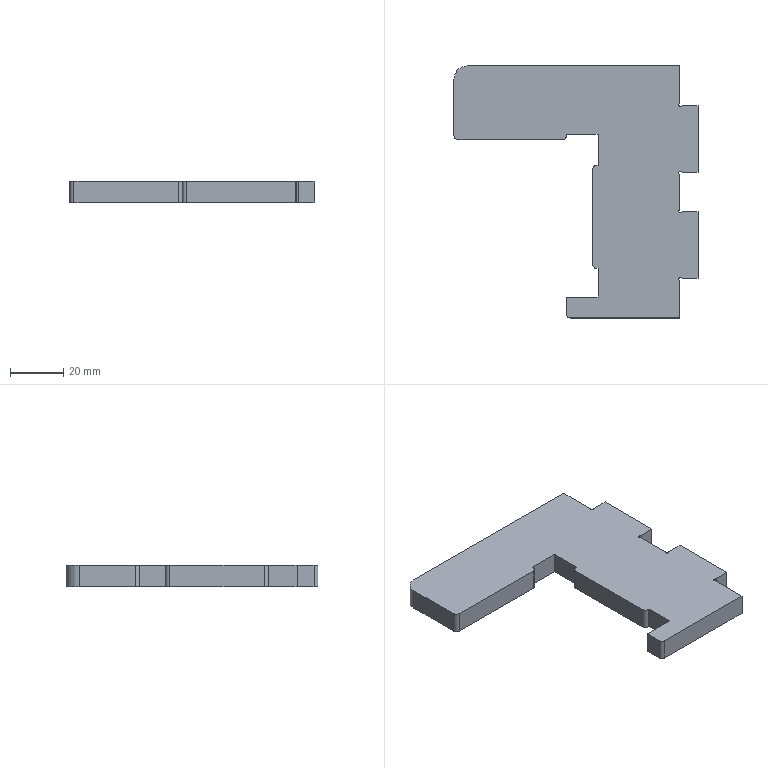Part | SolidWorks | features Fillet 2, FlatPattern 1, ICE 1, SMBaseFlange 1, SheetMetal 1 | 1 solid | 46 faces | box 92 x 95 x 8 mm | volume 39282 mm3 | plane 24 | cylinder 22 | commonest cylinder face diameters 3 x13 1 x8 10 x1
STEP:
#1=CARTESIAN_POINT('',(1503.95,-54.15,0.));
#2=VERTEX_POINT('',#1);
#3=CARTESIAN_POINT('',(1504.692,-53.713,0.));
#4=VERTEX_POINT('',#3);
#5=CARTESIAN_POINT('',(1504.45,-54.15,0.));
#6=DIRECTION('',(0.,0.,-1.));
#7=DIRECTION('',(-1.,0.,0.));
#8=AXIS2_PLACEMENT_3D('',#5,#6,#7);
#9=CIRCLE('',#8,0.5);
#10=EDGE_CURVE('',#2,#4,#9,.T.);
#11=ORIENTED_EDGE('',*,*,#10,.F.);
#12=CARTESIAN_POINT('',(1503.95,-54.15,-8.));
#13=VERTEX_POINT('',#12);
#14=CARTESIAN_POINT('',(1503.95,-54.15,-8.));
#15=DIRECTION('',(0.,0.,-1.));
#16=VECTOR('',#15,1000.);
#17=LINE('',#14,#16);
#18=EDGE_CURVE('',#2,#13,#17,.T.);
#19=ORIENTED_EDGE('',*,*,#18,.T.);
#20=CARTESIAN_POINT('',(1504.692,-53.713,-8.));
#21=VERTEX_POINT('',#20);
#22=CARTESIAN_POINT('',(1504.45,-54.15,-8.));
#23=DIRECTION('',(0.,0.,-1.));
#24=DIRECTION('',(-1.,0.,0.));
#25=AXIS2_PLACEMENT_3D('',#22,#23,#24);
#26=CIRCLE('',#25,0.5);
#27=EDGE_CURVE('',#13,#21,#26,.T.);
#28=ORIENTED_EDGE('',*,*,#27,.T.);
#29=CARTESIAN_POINT('',(1504.692,-53.713,-8.));
#30=DIRECTION('',(0.,0.,1.));
#31=VECTOR('',#30,1000.);
#32=LINE('',#29,#31);
#33=EDGE_CURVE('',#21,#4,#32,.T.);
#34=ORIENTED_EDGE('',*,*,#33,.T.);
#35=EDGE_LOOP('',(#11,#19,#28,#34));
#36=FACE_OUTER_BOUND('',#35,.T.);
#37=CARTESIAN_POINT('',(1504.45,-54.15,-8.));
#38=DIRECTION('',(0.,0.,-1.));
#39=DIRECTION('',(-1.,0.,0.));
#40=AXIS2_PLACEMENT_3D('',#37,#38,#39);
#41=CYLINDRICAL_SURFACE('',#40,0.5);
#42=ADVANCED_FACE('',(#36),#41,.F.);
#43=CARTESIAN_POINT('',(1503.95,11.35,0.));
#44=VERTEX_POINT('',#43);
#45=CARTESIAN_POINT('',(1504.013,11.592,0.));
#46=VERTEX_POINT('',#45);
#47=CARTESIAN_POINT('',(1504.45,11.35,0.));
#48=DIRECTION('',(0.,0.,-1.));
#49=DIRECTION('',(-1.,0.,0.));
#50=AXIS2_PLACEMENT_3D('',#47,#48,#49);
#51=CIRCLE('',#50,0.5);
#52=EDGE_CURVE('',#44,#46,#51,.T.);
#53=ORIENTED_EDGE('',*,*,#52,.F.);
#54=CARTESIAN_POINT('',(1503.95,11.35,-8.));
#55=VERTEX_POINT('',#54);
#56=CARTESIAN_POINT('',(1503.95,11.35,-8.));
#57=DIRECTION('',(0.,0.,-1.));
#58=VECTOR('',#57,1000.);
#59=LINE('',#56,#58);
#60=EDGE_CURVE('',#44,#55,#59,.T.);
#61=ORIENTED_EDGE('',*,*,#60,.T.);
#62=CARTESIAN_POINT('',(1504.013,11.592,-8.));
#63=VERTEX_POINT('',#62);
#64=CARTESIAN_POINT('',(1504.45,11.35,-8.));
#65=DIRECTION('',(0.,0.,-1.));
#66=DIRECTION('',(-1.,0.,0.));
#67=AXIS2_PLACEMENT_3D('',#64,#65,#66);
#68=CIRCLE('',#67,0.5);
#69=EDGE_CURVE('',#55,#63,#68,.T.);
#70=ORIENTED_EDGE('',*,*,#69,.T.);
#71=CARTESIAN_POINT('',(1504.013,11.592,-8.));
#72=DIRECTION('',(0.,0.,1.));
#73=VECTOR('',#72,1000.);
#74=LINE('',#71,#73);
#75=EDGE_CURVE('',#63,#46,#74,.T.);
#76=ORIENTED_EDGE('',*,*,#75,.T.);
#77=EDGE_LOOP('',(#53,#61,#70,#76));
#78=FACE_OUTER_BOUND('',#77,.T.);
#79=CARTESIAN_POINT('',(1504.45,11.35,-8.));
#80=DIRECTION('',(0.,0.,-1.));
#81=DIRECTION('',(-1.,0.,0.));
#82=AXIS2_PLACEMENT_3D('',#79,#80,#81);
#83=CYLINDRICAL_SURFACE('',#82,0.5);
#84=ADVANCED_FACE('',(#78),#83,.F.);
#85=CARTESIAN_POINT('',(1503.95,-14.15,0.));
#86=VERTEX_POINT('',#85);
#87=CARTESIAN_POINT('',(1504.692,-13.713,0.));
#88=VERTEX_POINT('',#87);
#89=CARTESIAN_POINT('',(1504.45,-14.15,0.));
#90=DIRECTION('',(0.,0.,-1.));
#91=DIRECTION('',(-1.,0.,0.));
#92=AXIS2_PLACEMENT_3D('',#89,#90,#91);
#93=CIRCLE('',#92,0.5);
#94=EDGE_CURVE('',#86,#88,#93,.T.);
#95=ORIENTED_EDGE('',*,*,#94,.F.);
#96=CARTESIAN_POINT('',(1503.95,-14.15,-8.));
#97=VERTEX_POINT('',#96);
#98=CARTESIAN_POINT('',(1503.95,-14.15,-8.));
#99=DIRECTION('',(0.,0.,-1.));
#100=VECTOR('',#99,1000.);
#101=LINE('',#98,#100);
#102=EDGE_CURVE('',#86,#97,#101,.T.);
#103=ORIENTED_EDGE('',*,*,#102,.T.);
#104=CARTESIAN_POINT('',(1504.692,-13.713,-8.));
#105=VERTEX_POINT('',#104);
#106=CARTESIAN_POINT('',(1504.45,-14.15,-8.));
#107=DIRECTION('',(0.,0.,-1.));
#108=DIRECTION('',(-1.,0.,0.));
#109=AXIS2_PLACEMENT_3D('',#106,#107,#108);
#110=CIRCLE('',#109,0.5);
#111=EDGE_CURVE('',#97,#105,#110,.T.);
#112=ORIENTED_EDGE('',*,*,#111,.T.);
#113=CARTESIAN_POINT('',(1504.692,-13.713,-8.));
#114=DIRECTION('',(0.,0.,1.));
#115=VECTOR('',#114,1000.);
#116=LINE('',#113,#115);
#117=EDGE_CURVE('',#105,#88,#116,.T.);
#118=ORIENTED_EDGE('',*,*,#117,.T.);
#119=EDGE_LOOP('',(#95,#103,#112,#118));
#120=FACE_OUTER_BOUND('',#119,.T.);
#121=CARTESIAN_POINT('',(1504.45,-14.15,-8.));
#122=DIRECTION('',(0.,0.,-1.));
#123=DIRECTION('',(-1.,0.,0.));
#124=AXIS2_PLACEMENT_3D('',#121,#122,#123);
#125=CYLINDRICAL_SURFACE('',#124,0.5);
#126=ADVANCED_FACE('',(#120),#125,.F.);
#127=CARTESIAN_POINT('',(1503.95,-28.653,0.));
#128=VERTEX_POINT('',#127);
#129=CARTESIAN_POINT('',(1504.013,-28.411,0.));
#130=VERTEX_POINT('',#129);
#131=CARTESIAN_POINT('',(1504.45,-28.653,0.));
#132=DIRECTION('',(0.,0.,-1.));
#133=DIRECTION('',(-1.,0.,0.));
#134=AXIS2_PLACEMENT_3D('',#131,#132,#133);
#135=CIRCLE('',#134,0.5);
#136=EDGE_CURVE('',#128,#130,#135,.T.);
#137=ORIENTED_EDGE('',*,*,#136,.F.);
#138=CARTESIAN_POINT('',(1503.95,-28.653,-8.));
#139=VERTEX_POINT('',#138);
#140=CARTESIAN_POINT('',(1503.95,-28.653,-8.));
#141=DIRECTION('',(0.,0.,-1.));
#142=VECTOR('',#141,1000.);
#143=LINE('',#140,#142);
#144=EDGE_CURVE('',#128,#139,#143,.T.);
#145=ORIENTED_EDGE('',*,*,#144,.T.);
#146=CARTESIAN_POINT('',(1504.013,-28.411,-8.));
#147=VERTEX_POINT('',#146);
#148=CARTESIAN_POINT('',(1504.45,-28.653,-8.));
#149=DIRECTION('',(0.,0.,-1.));
#150=DIRECTION('',(-1.,0.,0.));
#151=AXIS2_PLACEMENT_3D('',#148,#149,#150);
#152=CIRCLE('',#151,0.5);
#153=EDGE_CURVE('',#139,#147,#152,.T.);
#154=ORIENTED_EDGE('',*,*,#153,.T.);
#155=CARTESIAN_POINT('',(1504.013,-28.411,-8.));
#156=DIRECTION('',(0.,0.,1.));
#157=VECTOR('',#156,1000.);
#158=LINE('',#155,#157);
#159=EDGE_CURVE('',#147,#130,#158,.T.);
#160=ORIENTED_EDGE('',*,*,#159,.T.);
#161=EDGE_LOOP('',(#137,#145,#154,#160));
#162=FACE_OUTER_BOUND('',#161,.T.);
#163=CARTESIAN_POINT('',(1504.45,-28.653,-8.));
#164=DIRECTION('',(0.,0.,-1.));
#165=DIRECTION('',(-1.,0.,0.));
#166=AXIS2_PLACEMENT_3D('',#163,#164,#165);
#167=CYLINDRICAL_SURFACE('',#166,0.5);
#168=ADVANCED_FACE('',(#162),#167,.F.);
#169=CARTESIAN_POINT('',(1504.2,12.318,0.));
#170=VERTEX_POINT('',#169);
#171=CARTESIAN_POINT('',(1504.2,26.1,0.));
#172=VERTEX_POINT('',#171);
#173=CARTESIAN_POINT('',(1504.2,26.1,0.));
#174=DIRECTION('',(0.,1.,0.));
#175=VECTOR('',#174,1000.);
#176=LINE('',#173,#175);
#177=EDGE_CURVE('',#170,#172,#176,.T.);
#178=ORIENTED_EDGE('',*,*,#177,.F.);
#179=CARTESIAN_POINT('',(1504.2,12.318,-8.));
#180=VERTEX_POINT('',#179);
#181=CARTESIAN_POINT('',(1504.2,12.318,-8.));
#182=DIRECTION('',(0.,0.,-1.));
#183=VECTOR('',#182,1000.);
#184=LINE('',#181,#183);
#185=EDGE_CURVE('',#170,#180,#184,.T.);
#186=ORIENTED_EDGE('',*,*,#185,.T.);
#187=CARTESIAN_POINT('',(1504.2,26.1,-8.));
#188=VERTEX_POINT('',#187);
#189=CARTESIAN_POINT('',(1504.2,26.1,-8.));
#190=DIRECTION('',(0.,1.,0.));
#191=VECTOR('',#190,1000.);
#192=LINE('',#189,#191);
#193=EDGE_CURVE('',#180,#188,#192,.T.);
#194=ORIENTED_EDGE('',*,*,#193,.T.);
#195=CARTESIAN_POINT('',(1504.2,26.1,-8.));
#196=DIRECTION('',(0.,0.,1.));
#197=VECTOR('',#196,1000.);
#198=LINE('',#195,#197);
#199=EDGE_CURVE('',#188,#172,#198,.T.);
#200=ORIENTED_EDGE('',*,*,#199,.T.);
#201=EDGE_LOOP('',(#178,#186,#194,#200));
#202=FACE_OUTER_BOUND('',#201,.T.);
#203=CARTESIAN_POINT('',(1504.2,26.1,-8.));
#204=DIRECTION('',(1.,0.,0.));
#205=DIRECTION('',(0.,0.,-1.));
#206=AXIS2_PLACEMENT_3D('',#203,#204,#205);
#207=PLANE('',#206);
#208=ADVANCED_FACE('',(#202),#207,.T.);
#209=CARTESIAN_POINT('',(1511.2,11.1,-8.));
#210=VERTEX_POINT('',#209);
#211=CARTESIAN_POINT('',(1505.418,11.1,-8.));
#212=VERTEX_POINT('',#211);
#213=CARTESIAN_POINT('',(1511.2,11.1,-8.));
#214=DIRECTION('',(-1.,0.,0.));
#215=VECTOR('',#214,1000.);
#216=LINE('',#213,#215);
#217=EDGE_CURVE('',#210,#212,#216,.T.);
#218=ORIENTED_EDGE('',*,*,#217,.T.);
#219=CARTESIAN_POINT('',(1505.418,11.1,0.));
#220=VERTEX_POINT('',#219);
#221=CARTESIAN_POINT('',(1505.418,11.1,-8.));
#222=DIRECTION('',(0.,0.,1.));
#223=VECTOR('',#222,1000.);
#224=LINE('',#221,#223);
#225=EDGE_CURVE('',#212,#220,#224,.T.);
#226=ORIENTED_EDGE('',*,*,#225,.T.);
#227=CARTESIAN_POINT('',(1511.2,11.1,0.));
#228=VERTEX_POINT('',#227);
#229=CARTESIAN_POINT('',(1511.2,11.1,0.));
#230=DIRECTION('',(-1.,0.,0.));
#231=VECTOR('',#230,1000.);
#232=LINE('',#229,#231);
#233=EDGE_CURVE('',#228,#220,#232,.T.);
#234=ORIENTED_EDGE('',*,*,#233,.F.);
#235=CARTESIAN_POINT('',(1511.2,11.1,-8.));
#236=DIRECTION('',(0.,0.,1.));
#237=VECTOR('',#236,1000.);
#238=LINE('',#235,#237);
#239=EDGE_CURVE('',#210,#228,#238,.T.);
#240=ORIENTED_EDGE('',*,*,#239,.F.);
#241=EDGE_LOOP('',(#218,#226,#234,#240));
#242=FACE_OUTER_BOUND('',#241,.T.);
#243=CARTESIAN_POINT('',(1511.2,11.1,-8.));
#244=DIRECTION('',(0.,1.,0.));
#245=DIRECTION('',(0.,0.,1.));
#246=AXIS2_PLACEMENT_3D('',#243,#244,#245);
#247=PLANE('',#246);
#248=ADVANCED_FACE('',(#242),#247,.T.);
#249=CARTESIAN_POINT('',(1505.418,-13.9,0.));
#250=VERTEX_POINT('',#249);
#251=CARTESIAN_POINT('',(1511.2,-13.9,0.));
#252=VERTEX_POINT('',#251);
#253=CARTESIAN_POINT('',(1504.2,-13.9,0.));
#254=DIRECTION('',(1.,0.,0.));
#255=VECTOR('',#254,1000.);
#256=LINE('',#253,#255);
#257=EDGE_CURVE('',#250,#252,#256,.T.);
#258=ORIENTED_EDGE('',*,*,#257,.F.);
#259=CARTESIAN_POINT('',(1505.418,-13.9,-8.));
#260=VERTEX_POINT('',#259);
#261=CARTESIAN_POINT('',(1505.418,-13.9,-8.));
#262=DIRECTION('',(0.,0.,-1.));
#263=VECTOR('',#262,1000.);
#264=LINE('',#261,#263);
#265=EDGE_CURVE('',#250,#260,#264,.T.);
#266=ORIENTED_EDGE('',*,*,#265,.T.);
#267=CARTESIAN_POINT('',(1511.2,-13.9,-8.));
#268=VERTEX_POINT('',#267);
#269=CARTESIAN_POINT('',(1504.2,-13.9,-8.));
#270=DIRECTION('',(1.,0.,0.));
#271=VECTOR('',#270,1000.);
#272=LINE('',#269,#271);
#273=EDGE_CURVE('',#260,#268,#272,.T.);
#274=ORIENTED_EDGE('',*,*,#273,.T.);
#275=CARTESIAN_POINT('',(1511.2,-13.9,-8.));
#276=DIRECTION('',(0.,0.,1.));
#277=VECTOR('',#276,1000.);
#278=LINE('',#275,#277);
#279=EDGE_CURVE('',#268,#252,#278,.T.);
#280=ORIENTED_EDGE('',*,*,#279,.T.);
#281=EDGE_LOOP('',(#258,#266,#274,#280));
#282=FACE_OUTER_BOUND('',#281,.T.);
#283=CARTESIAN_POINT('',(1504.2,-13.9,-8.));
#284=DIRECTION('',(0.,-1.,0.));
#285=DIRECTION('',(0.,0.,-1.));
#286=AXIS2_PLACEMENT_3D('',#283,#284,#285);
#287=PLANE('',#286);
#288=ADVANCED_FACE('',(#282),#287,.T.);
#289=CARTESIAN_POINT('',(1504.2,-27.685,0.));
#290=VERTEX_POINT('',#289);
#291=CARTESIAN_POINT('',(1504.2,-15.118,0.));
#292=VERTEX_POINT('',#291);
#293=CARTESIAN_POINT('',(1504.2,-13.9,0.));
#294=DIRECTION('',(0.,1.,0.));
#295=VECTOR('',#294,1000.);
#296=LINE('',#293,#295);
#297=EDGE_CURVE('',#290,#292,#296,.T.);
#298=ORIENTED_EDGE('',*,*,#297,.F.);
#299=CARTESIAN_POINT('',(1504.2,-27.685,-8.));
#300=VERTEX_POINT('',#299);
#301=CARTESIAN_POINT('',(1504.2,-27.685,-8.));
#302=DIRECTION('',(0.,0.,-1.));
#303=VECTOR('',#302,1000.);
#304=LINE('',#301,#303);
#305=EDGE_CURVE('',#290,#300,#304,.T.);
#306=ORIENTED_EDGE('',*,*,#305,.T.);
#307=CARTESIAN_POINT('',(1504.2,-15.118,-8.));
#308=VERTEX_POINT('',#307);
#309=CARTESIAN_POINT('',(1504.2,-13.9,-8.));
#310=DIRECTION('',(0.,1.,0.));
#311=VECTOR('',#310,1000.);
#312=LINE('',#309,#311);
#313=EDGE_CURVE('',#300,#308,#312,.T.);
#314=ORIENTED_EDGE('',*,*,#313,.T.);
#315=CARTESIAN_POINT('',(1504.2,-15.118,-8.));
#316=DIRECTION('',(0.,0.,1.));
#317=VECTOR('',#316,1000.);
#318=LINE('',#315,#317);
#319=EDGE_CURVE('',#308,#292,#318,.T.);
#320=ORIENTED_EDGE('',*,*,#319,.T.);
#321=EDGE_LOOP('',(#298,#306,#314,#320));
#322=FACE_OUTER_BOUND('',#321,.T.);
#323=CARTESIAN_POINT('',(1504.2,-13.9,-8.));
#324=DIRECTION('',(1.,0.,0.));
#325=DIRECTION('',(0.,0.,-1.));
#326=AXIS2_PLACEMENT_3D('',#323,#324,#325);
#327=PLANE('',#326);
#328=ADVANCED_FACE('',(#322),#327,.T.);
#329=CARTESIAN_POINT('',(1511.2,-28.9,-8.));
#330=VERTEX_POINT('',#329);
#331=CARTESIAN_POINT('',(1505.423,-28.9,-8.));
#332=VERTEX_POINT('',#331);
#333=CARTESIAN_POINT('',(1511.2,-28.9,-8.));
#334=DIRECTION('',(-1.,0.,0.));
#335=VECTOR('',#334,1000.);
#336=LINE('',#333,#335);
#337=EDGE_CURVE('',#330,#332,#336,.T.);
#338=ORIENTED_EDGE('',*,*,#337,.T.);
#339=CARTESIAN_POINT('',(1505.423,-28.9,0.));
#340=VERTEX_POINT('',#339);
#341=CARTESIAN_POINT('',(1505.423,-28.9,-8.));
#342=DIRECTION('',(0.,0.,1.));
#343=VECTOR('',#342,1000.);
#344=LINE('',#341,#343);
#345=EDGE_CURVE('',#332,#340,#344,.T.);
#346=ORIENTED_EDGE('',*,*,#345,.T.);
#347=CARTESIAN_POINT('',(1511.2,-28.9,0.));
#348=VERTEX_POINT('',#347);
#349=CARTESIAN_POINT('',(1511.2,-28.9,0.));
#350=DIRECTION('',(-1.,0.,0.));
#351=VECTOR('',#350,1000.);
#352=LINE('',#349,#351);
#353=EDGE_CURVE('',#348,#340,#352,.T.);
#354=ORIENTED_EDGE('',*,*,#353,.F.);
#355=CARTESIAN_POINT('',(1511.2,-28.9,-8.));
#356=DIRECTION('',(0.,0.,1.));
#357=VECTOR('',#356,1000.);
#358=LINE('',#355,#357);
#359=EDGE_CURVE('',#330,#348,#358,.T.);
#360=ORIENTED_EDGE('',*,*,#359,.F.);
#361=EDGE_LOOP('',(#338,#346,#354,#360));
#362=FACE_OUTER_BOUND('',#361,.T.);
#363=CARTESIAN_POINT('',(1511.2,-28.9,-8.));
#364=DIRECTION('',(0.,1.,0.));
#365=DIRECTION('',(0.,0.,1.));
#366=AXIS2_PLACEMENT_3D('',#363,#364,#365);
#367=PLANE('',#366);
#368=ADVANCED_FACE('',(#362),#367,.T.);
#369=CARTESIAN_POINT('',(1505.418,-53.9,0.));
#370=VERTEX_POINT('',#369);
#371=CARTESIAN_POINT('',(1511.2,-53.9,0.));
#372=VERTEX_POINT('',#371);
#373=CARTESIAN_POINT('',(1511.2,-53.9,0.));
#374=DIRECTION('',(1.,0.,0.));
#375=VECTOR('',#374,1000.);
#376=LINE('',#373,#375);
#377=EDGE_CURVE('',#370,#372,#376,.T.);
#378=ORIENTED_EDGE('',*,*,#377,.F.);
#379=CARTESIAN_POINT('',(1505.418,-53.9,-8.));
#380=VERTEX_POINT('',#379);
#381=CARTESIAN_POINT('',(1505.418,-53.9,-8.));
#382=DIRECTION('',(0.,0.,-1.));
#383=VECTOR('',#382,1000.);
#384=LINE('',#381,#383);
#385=EDGE_CURVE('',#370,#380,#384,.T.);
#386=ORIENTED_EDGE('',*,*,#385,.T.);
#387=CARTESIAN_POINT('',(1511.2,-53.9,-8.));
#388=VERTEX_POINT('',#387);
#389=CARTESIAN_POINT('',(1511.2,-53.9,-8.));
#390=DIRECTION('',(1.,0.,0.));
#391=VECTOR('',#390,1000.);
#392=LINE('',#389,#391);
#393=EDGE_CURVE('',#380,#388,#392,.T.);
#394=ORIENTED_EDGE('',*,*,#393,.T.);
#395=CARTESIAN_POINT('',(1511.2,-53.9,-8.));
#396=DIRECTION('',(0.,0.,1.));
#397=VECTOR('',#396,1000.);
#398=LINE('',#395,#397);
#399=EDGE_CURVE('',#388,#372,#398,.T.);
#400=ORIENTED_EDGE('',*,*,#399,.T.);
#401=EDGE_LOOP('',(#378,#386,#394,#400));
#402=FACE_OUTER_BOUND('',#401,.T.);
#403=CARTESIAN_POINT('',(1511.2,-53.9,-8.));
#404=DIRECTION('',(0.,-1.,0.));
#405=DIRECTION('',(1.,0.,0.));
#406=AXIS2_PLACEMENT_3D('',#403,#404,#405);
#407=PLANE('',#406);
#408=ADVANCED_FACE('',(#402),#407,.T.);
#409=CARTESIAN_POINT('',(1504.2,-68.9,-8.));
#410=VERTEX_POINT('',#409);
#411=CARTESIAN_POINT('',(1504.2,-55.118,-8.));
#412=VERTEX_POINT('',#411);
#413=CARTESIAN_POINT('',(1504.2,-53.9,-8.));
#414=DIRECTION('',(0.,1.,0.));
#415=VECTOR('',#414,1000.);
#416=LINE('',#413,#415);
#417=EDGE_CURVE('',#410,#412,#416,.T.);
#418=ORIENTED_EDGE('',*,*,#417,.T.);
#419=CARTESIAN_POINT('',(1504.2,-55.118,0.));
#420=VERTEX_POINT('',#419);
#421=CARTESIAN_POINT('',(1504.2,-55.118,-8.));
#422=DIRECTION('',(0.,0.,1.));
#423=VECTOR('',#422,1000.);
#424=LINE('',#421,#423);
#425=EDGE_CURVE('',#412,#420,#424,.T.);
#426=ORIENTED_EDGE('',*,*,#425,.T.);
#427=CARTESIAN_POINT('',(1504.2,-68.9,0.));
#428=VERTEX_POINT('',#427);
#429=CARTESIAN_POINT('',(1504.2,-53.9,0.));
#430=DIRECTION('',(0.,1.,0.));
#431=VECTOR('',#430,1000.);
#432=LINE('',#429,#431);
#433=EDGE_CURVE('',#428,#420,#432,.T.);
#434=ORIENTED_EDGE('',*,*,#433,.F.);
#435=CARTESIAN_POINT('',(1504.2,-68.9,-8.));
#436=DIRECTION('',(0.,0.,1.));
#437=VECTOR('',#436,1000.);
#438=LINE('',#435,#437);
#439=EDGE_CURVE('',#410,#428,#438,.T.);
#440=ORIENTED_EDGE('',*,*,#439,.F.);
#441=EDGE_LOOP('',(#418,#426,#434,#440));
#442=FACE_OUTER_BOUND('',#441,.T.);
#443=CARTESIAN_POINT('',(1504.2,-53.9,-8.));
#444=DIRECTION('',(1.,0.,0.));
#445=DIRECTION('',(0.,0.,-1.));
#446=AXIS2_PLACEMENT_3D('',#443,#444,#445);
#447=PLANE('',#446);
#448=ADVANCED_FACE('',(#442),#447,.T.);
#449=CARTESIAN_POINT('',(1420.7,-1.6,-8.));
#450=VERTEX_POINT('',#449);
#451=CARTESIAN_POINT('',(1460.2,-1.6,-8.));
#452=VERTEX_POINT('',#451);
#453=CARTESIAN_POINT('',(1461.7,-1.6,-8.));
#454=DIRECTION('',(1.,0.,0.));
#455=VECTOR('',#454,1000.);
#456=LINE('',#453,#455);
#457=EDGE_CURVE('',#450,#452,#456,.T.);
#458=ORIENTED_EDGE('',*,*,#457,.T.);
#459=CARTESIAN_POINT('',(1460.2,-1.6,0.));
#460=VERTEX_POINT('',#459);
#461=CARTESIAN_POINT('',(1460.2,-1.6,-8.));
#462=DIRECTION('',(0.,0.,1.));
#463=VECTOR('',#462,1000.);
#464=LINE('',#461,#463);
#465=EDGE_CURVE('',#452,#460,#464,.T.);
#466=ORIENTED_EDGE('',*,*,#465,.T.);
#467=CARTESIAN_POINT('',(1420.7,-1.6,0.));
#468=VERTEX_POINT('',#467);
#469=CARTESIAN_POINT('',(1461.7,-1.6,0.));
#470=DIRECTION('',(1.,0.,0.));
#471=VECTOR('',#470,1000.);
#472=LINE('',#469,#471);
#473=EDGE_CURVE('',#468,#460,#472,.T.);
#474=ORIENTED_EDGE('',*,*,#473,.F.);
#475=CARTESIAN_POINT('',(1420.7,-1.6,-8.));
#476=DIRECTION('',(0.,0.,-1.));
#477=VECTOR('',#476,1000.);
#478=LINE('',#475,#477);
#479=EDGE_CURVE('',#468,#450,#478,.T.);
#480=ORIENTED_EDGE('',*,*,#479,.T.);
#481=EDGE_LOOP('',(#458,#466,#474,#480));
#482=FACE_OUTER_BOUND('',#481,.T.);
#483=CARTESIAN_POINT('',(1461.7,-1.6,-8.));
#484=DIRECTION('',(0.,-1.,0.));
#485=DIRECTION('',(0.,0.,-1.));
#486=AXIS2_PLACEMENT_3D('',#483,#484,#485);
#487=PLANE('',#486);
#488=ADVANCED_FACE('',(#482),#487,.T.);
#489=CARTESIAN_POINT('',(1419.2,21.1,0.));
#490=VERTEX_POINT('',#489);
#491=CARTESIAN_POINT('',(1419.2,-0.1,0.));
#492=VERTEX_POINT('',#491);
#493=CARTESIAN_POINT('',(1419.2,-1.6,0.));
#494=DIRECTION('',(0.,-1.,0.));
#495=VECTOR('',#494,1000.);
#496=LINE('',#493,#495);
#497=EDGE_CURVE('',#490,#492,#496,.T.);
#498=ORIENTED_EDGE('',*,*,#497,.F.);
#499=CARTESIAN_POINT('',(1419.2,21.1,-8.));
#500=VERTEX_POINT('',#499);
#501=CARTESIAN_POINT('',(1419.2,21.1,-8.));
#502=DIRECTION('',(0.,0.,-1.));
#503=VECTOR('',#502,1000.);
#504=LINE('',#501,#503);
#505=EDGE_CURVE('',#490,#500,#504,.T.);
#506=ORIENTED_EDGE('',*,*,#505,.T.);
#507=CARTESIAN_POINT('',(1419.2,-0.1,-8.));
#508=VERTEX_POINT('',#507);
#509=CARTESIAN_POINT('',(1419.2,-1.6,-8.));
#510=DIRECTION('',(0.,-1.,0.));
#511=VECTOR('',#510,1000.);
#512=LINE('',#509,#511);
#513=EDGE_CURVE('',#500,#508,#512,.T.);
#514=ORIENTED_EDGE('',*,*,#513,.T.);
#515=CARTESIAN_POINT('',(1419.2,-0.1,-8.));
#516=DIRECTION('',(0.,0.,1.));
#517=VECTOR('',#516,1000.);
#518=LINE('',#515,#517);
#519=EDGE_CURVE('',#508,#492,#518,.T.);
#520=ORIENTED_EDGE('',*,*,#519,.T.);
#521=EDGE_LOOP('',(#498,#506,#514,#520));
#522=FACE_OUTER_BOUND('',#521,.T.);
#523=CARTESIAN_POINT('',(1419.2,-1.6,-8.));
#524=DIRECTION('',(-1.,0.,0.));
#525=DIRECTION('',(0.,0.,1.));
#526=AXIS2_PLACEMENT_3D('',#523,#524,#525);
#527=PLANE('',#526);
#528=ADVANCED_FACE('',(#522),#527,.T.);
#529=CARTESIAN_POINT('',(1424.2,26.1,-8.));
#530=VERTEX_POINT('',#529);
#531=CARTESIAN_POINT('',(1419.2,26.1,-8.));
#532=DIRECTION('',(-1.,0.,0.));
#533=VECTOR('',#532,1000.);
#534=LINE('',#531,#533);
#535=EDGE_CURVE('',#188,#530,#534,.T.);
#536=ORIENTED_EDGE('',*,*,#535,.T.);
#537=CARTESIAN_POINT('',(1424.2,26.1,0.));
#538=VERTEX_POINT('',#537);
#539=CARTESIAN_POINT('',(1424.2,26.1,-8.));
#540=DIRECTION('',(0.,0.,1.));
#541=VECTOR('',#540,1000.);
#542=LINE('',#539,#541);
#543=EDGE_CURVE('',#530,#538,#542,.T.);
#544=ORIENTED_EDGE('',*,*,#543,.T.);
#545=CARTESIAN_POINT('',(1419.2,26.1,0.));
#546=DIRECTION('',(-1.,0.,0.));
#547=VECTOR('',#546,1000.);
#548=LINE('',#545,#547);
#549=EDGE_CURVE('',#172,#538,#548,.T.);
#550=ORIENTED_EDGE('',*,*,#549,.F.);
#551=ORIENTED_EDGE('',*,*,#199,.F.);
#552=EDGE_LOOP('',(#536,#544,#550,#551));
#553=FACE_OUTER_BOUND('',#552,.T.);
#554=CARTESIAN_POINT('',(1419.2,26.1,-8.));
#555=DIRECTION('',(0.,1.,0.));
#556=DIRECTION('',(0.,0.,1.));
#557=AXIS2_PLACEMENT_3D('',#554,#555,#556);
#558=PLANE('',#557);
#559=ADVANCED_FACE('',(#553),#558,.T.);
#560=CARTESIAN_POINT('',(1511.2,-13.9,0.));
#561=DIRECTION('',(0.,1.,0.));
#562=VECTOR('',#561,1000.);
#563=LINE('',#560,#562);
#564=EDGE_CURVE('',#252,#228,#563,.T.);
#565=ORIENTED_EDGE('',*,*,#564,.F.);
#566=ORIENTED_EDGE('',*,*,#279,.F.);
#567=CARTESIAN_POINT('',(1511.2,-13.9,-8.));
#568=DIRECTION('',(0.,1.,0.));
#569=VECTOR('',#568,1000.);
#570=LINE('',#567,#569);
#571=EDGE_CURVE('',#268,#210,#570,.T.);
#572=ORIENTED_EDGE('',*,*,#571,.T.);
#573=ORIENTED_EDGE('',*,*,#239,.T.);
#574=EDGE_LOOP('',(#565,#566,#572,#573));
#575=FACE_OUTER_BOUND('',#574,.T.);
#576=CARTESIAN_POINT('',(1511.2,-13.9,-8.));
#577=DIRECTION('',(1.,0.,0.));
#578=DIRECTION('',(0.,0.,-1.));
#579=AXIS2_PLACEMENT_3D('',#576,#577,#578);
#580=PLANE('',#579);
#581=ADVANCED_FACE('',(#575),#580,.T.);
#582=CARTESIAN_POINT('',(1511.2,-28.9,0.));
#583=DIRECTION('',(0.,1.,0.));
#584=VECTOR('',#583,1000.);
#585=LINE('',#582,#584);
#586=EDGE_CURVE('',#372,#348,#585,.T.);
#587=ORIENTED_EDGE('',*,*,#586,.F.);
#588=ORIENTED_EDGE('',*,*,#399,.F.);
#589=CARTESIAN_POINT('',(1511.2,-28.9,-8.));
#590=DIRECTION('',(0.,1.,0.));
#591=VECTOR('',#590,1000.);
#592=LINE('',#589,#591);
#593=EDGE_CURVE('',#388,#330,#592,.T.);
#594=ORIENTED_EDGE('',*,*,#593,.T.);
#595=ORIENTED_EDGE('',*,*,#359,.T.);
#596=EDGE_LOOP('',(#587,#588,#594,#595));
#597=FACE_OUTER_BOUND('',#596,.T.);
#598=CARTESIAN_POINT('',(1511.2,-28.9,-8.));
#599=DIRECTION('',(1.,0.,0.));
#600=DIRECTION('',(0.,1.,0.));
#601=AXIS2_PLACEMENT_3D('',#598,#599,#600);
#602=PLANE('',#601);
#603=ADVANCED_FACE('',(#597),#602,.T.);
#604=CARTESIAN_POINT('',(1463.,-68.9,0.));
#605=VERTEX_POINT('',#604);
#606=CARTESIAN_POINT('',(1504.2,-68.9,0.));
#607=DIRECTION('',(1.,0.,0.));
#608=VECTOR('',#607,1000.);
#609=LINE('',#606,#608);
#610=EDGE_CURVE('',#605,#428,#609,.T.);
#611=ORIENTED_EDGE('',*,*,#610,.F.);
#612=CARTESIAN_POINT('',(1463.,-68.9,-8.));
#613=VERTEX_POINT('',#612);
#614=CARTESIAN_POINT('',(1463.,-68.9,-8.));
#615=DIRECTION('',(0.,0.,-1.));
#616=VECTOR('',#615,1000.);
#617=LINE('',#614,#616);
#618=EDGE_CURVE('',#605,#613,#617,.T.);
#619=ORIENTED_EDGE('',*,*,#618,.T.);
#620=CARTESIAN_POINT('',(1504.2,-68.9,-8.));
#621=DIRECTION('',(1.,0.,0.));
#622=VECTOR('',#621,1000.);
#623=LINE('',#620,#622);
#624=EDGE_CURVE('',#613,#410,#623,.T.);
#625=ORIENTED_EDGE('',*,*,#624,.T.);
#626=ORIENTED_EDGE('',*,*,#439,.T.);
#627=EDGE_LOOP('',(#611,#619,#625,#626));
#628=FACE_OUTER_BOUND('',#627,.T.);
#629=CARTESIAN_POINT('',(1504.2,-68.9,-8.));
#630=DIRECTION('',(0.,-1.,0.));
#631=DIRECTION('',(0.,0.,-1.));
#632=AXIS2_PLACEMENT_3D('',#629,#630,#631);
#633=PLANE('',#632);
#634=ADVANCED_FACE('',(#628),#633,.T.);
#635=CARTESIAN_POINT('',(1461.5,-61.,-8.));
#636=VERTEX_POINT('',#635);
#637=CARTESIAN_POINT('',(1461.5,-67.4,-8.));
#638=VERTEX_POINT('',#637);
#639=CARTESIAN_POINT('',(1461.5,-61.,-8.));
#640=DIRECTION('',(0.,-1.,0.));
#641=VECTOR('',#640,1000.);
#642=LINE('',#639,#641);
#643=EDGE_CURVE('',#636,#638,#642,.T.);
#644=ORIENTED_EDGE('',*,*,#643,.T.);
#645=CARTESIAN_POINT('',(1461.5,-67.4,0.));
#646=VERTEX_POINT('',#645);
#647=CARTESIAN_POINT('',(1461.5,-67.4,-8.));
#648=DIRECTION('',(0.,0.,1.));
#649=VECTOR('',#648,1000.);
#650=LINE('',#647,#649);
#651=EDGE_CURVE('',#638,#646,#650,.T.);
#652=ORIENTED_EDGE('',*,*,#651,.T.);
#653=CARTESIAN_POINT('',(1461.5,-61.,0.));
#654=VERTEX_POINT('',#653);
#655=CARTESIAN_POINT('',(1461.5,-61.,0.));
#656=DIRECTION('',(0.,-1.,0.));
#657=VECTOR('',#656,1000.);
#658=LINE('',#655,#657);
#659=EDGE_CURVE('',#654,#646,#658,.T.);
#660=ORIENTED_EDGE('',*,*,#659,.F.);
#661=CARTESIAN_POINT('',(1461.5,-61.,-8.));
#662=DIRECTION('',(0.,0.,1.));
#663=VECTOR('',#662,1000.);
#664=LINE('',#661,#663);
#665=EDGE_CURVE('',#636,#654,#664,.T.);
#666=ORIENTED_EDGE('',*,*,#665,.F.);
#667=EDGE_LOOP('',(#644,#652,#660,#666));
#668=FACE_OUTER_BOUND('',#667,.T.);
#669=CARTESIAN_POINT('',(1461.5,-61.,-8.));
#670=DIRECTION('',(-1.,0.,0.));
#671=DIRECTION('',(0.,0.,1.));
#672=AXIS2_PLACEMENT_3D('',#669,#670,#671);
#673=PLANE('',#672);
#674=ADVANCED_FACE('',(#668),#673,.T.);
#675=CARTESIAN_POINT('',(1473.5,-61.,0.));
#676=VERTEX_POINT('',#675);
#677=CARTESIAN_POINT('',(1473.5,-61.,0.));
#678=DIRECTION('',(-1.,0.,0.));
#679=VECTOR('',#678,1000.);
#680=LINE('',#677,#679);
#681=EDGE_CURVE('',#676,#654,#680,.T.);
#682=ORIENTED_EDGE('',*,*,#681,.F.);
#683=CARTESIAN_POINT('',(1473.5,-61.,-8.));
#684=VERTEX_POINT('',#683);
#685=CARTESIAN_POINT('',(1473.5,-61.,-8.));
#686=DIRECTION('',(0.,0.,1.));
#687=VECTOR('',#686,1000.);
#688=LINE('',#685,#687);
#689=EDGE_CURVE('',#684,#676,#688,.T.);
#690=ORIENTED_EDGE('',*,*,#689,.F.);
#691=CARTESIAN_POINT('',(1473.5,-61.,-8.));
#692=DIRECTION('',(-1.,0.,0.));
#693=VECTOR('',#692,1000.);
#694=LINE('',#691,#693);
#695=EDGE_CURVE('',#684,#636,#694,.T.);
#696=ORIENTED_EDGE('',*,*,#695,.T.);
#697=ORIENTED_EDGE('',*,*,#665,.T.);
#698=EDGE_LOOP('',(#682,#690,#696,#697));
#699=FACE_OUTER_BOUND('',#698,.T.);
#700=CARTESIAN_POINT('',(1473.5,-61.,-8.));
#701=DIRECTION('',(0.,1.,0.));
#702=DIRECTION('',(0.,0.,1.));
#703=AXIS2_PLACEMENT_3D('',#700,#701,#702);
#704=PLANE('',#703);
#705=ADVANCED_FACE('',(#699),#704,.T.);
#706=CARTESIAN_POINT('',(1473.5,-50.2,0.));
#707=VERTEX_POINT('',#706);
#708=CARTESIAN_POINT('',(1473.5,-61.,0.));
#709=DIRECTION('',(0.,-1.,0.));
#710=VECTOR('',#709,1000.);
#711=LINE('',#708,#710);
#712=EDGE_CURVE('',#707,#676,#711,.T.);
#713=ORIENTED_EDGE('',*,*,#712,.F.);
#714=CARTESIAN_POINT('',(1473.5,-50.2,-8.));
#715=VERTEX_POINT('',#714);
#716=CARTESIAN_POINT('',(1473.5,-50.2,-8.));
#717=DIRECTION('',(0.,0.,1.));
#718=VECTOR('',#717,1000.);
#719=LINE('',#716,#718);
#720=EDGE_CURVE('',#715,#707,#719,.T.);
#721=ORIENTED_EDGE('',*,*,#720,.F.);
#722=CARTESIAN_POINT('',(1473.5,-61.,-8.));
#723=DIRECTION('',(0.,-1.,0.));
#724=VECTOR('',#723,1000.);
#725=LINE('',#722,#724);
#726=EDGE_CURVE('',#715,#684,#725,.T.);
#727=ORIENTED_EDGE('',*,*,#726,.T.);
#728=ORIENTED_EDGE('',*,*,#689,.T.);
#729=EDGE_LOOP('',(#713,#721,#727,#728));
#730=FACE_OUTER_BOUND('',#729,.T.);
#731=CARTESIAN_POINT('',(1473.5,-61.,-8.));
#732=DIRECTION('',(-1.,0.,0.));
#733=DIRECTION('',(0.,0.,1.));
#734=AXIS2_PLACEMENT_3D('',#731,#732,#733);
#735=PLANE('',#734);
#736=ADVANCED_FACE('',(#730),#735,.T.);
#737=CARTESIAN_POINT('',(1473.,-50.2,0.));
#738=VERTEX_POINT('',#737);
#739=CARTESIAN_POINT('',(1473.5,-50.2,0.));
#740=DIRECTION('',(1.,0.,0.));
#741=VECTOR('',#740,1000.);
#742=LINE('',#739,#741);
#743=EDGE_CURVE('',#738,#707,#742,.T.);
#744=ORIENTED_EDGE('',*,*,#743,.F.);
#745=CARTESIAN_POINT('',(1473.,-50.2,-8.));
#746=VERTEX_POINT('',#745);
#747=CARTESIAN_POINT('',(1473.,-50.2,-8.));
#748=DIRECTION('',(0.,0.,-1.));
#749=VECTOR('',#748,1000.);
#750=LINE('',#747,#749);
#751=EDGE_CURVE('',#738,#746,#750,.T.);
#752=ORIENTED_EDGE('',*,*,#751,.T.);
#753=CARTESIAN_POINT('',(1473.5,-50.2,-8.));
#754=DIRECTION('',(1.,0.,0.));
#755=VECTOR('',#754,1000.);
#756=LINE('',#753,#755);
#757=EDGE_CURVE('',#746,#715,#756,.T.);
#758=ORIENTED_EDGE('',*,*,#757,.T.);
#759=ORIENTED_EDGE('',*,*,#720,.T.);
#760=EDGE_LOOP('',(#744,#752,#758,#759));
#761=FACE_OUTER_BOUND('',#760,.T.);
#762=CARTESIAN_POINT('',(1473.5,-50.2,-8.));
#763=DIRECTION('',(0.,-1.,0.));
#764=DIRECTION('',(0.,0.,-1.));
#765=AXIS2_PLACEMENT_3D('',#762,#763,#764);
#766=PLANE('',#765);
#767=ADVANCED_FACE('',(#761),#766,.T.);
#768=CARTESIAN_POINT('',(1471.5,-12.9,-8.));
#769=VERTEX_POINT('',#768);
#770=CARTESIAN_POINT('',(1471.5,-48.7,-8.));
#771=VERTEX_POINT('',#770);
#772=CARTESIAN_POINT('',(1471.5,-50.2,-8.));
#773=DIRECTION('',(0.,-1.,0.));
#774=VECTOR('',#773,1000.);
#775=LINE('',#772,#774);
#776=EDGE_CURVE('',#769,#771,#775,.T.);
#777=ORIENTED_EDGE('',*,*,#776,.T.);
#778=CARTESIAN_POINT('',(1471.5,-48.7,0.));
#779=VERTEX_POINT('',#778);
#780=CARTESIAN_POINT('',(1471.5,-48.7,-8.));
#781=DIRECTION('',(0.,0.,1.));
#782=VECTOR('',#781,1000.);
#783=LINE('',#780,#782);
#784=EDGE_CURVE('',#771,#779,#783,.T.);
#785=ORIENTED_EDGE('',*,*,#784,.T.);
#786=CARTESIAN_POINT('',(1471.5,-12.9,0.));
#787=VERTEX_POINT('',#786);
#788=CARTESIAN_POINT('',(1471.5,-50.2,0.));
#789=DIRECTION('',(0.,-1.,0.));
#790=VECTOR('',#789,1000.);
#791=LINE('',#788,#790);
#792=EDGE_CURVE('',#787,#779,#791,.T.);
#793=ORIENTED_EDGE('',*,*,#792,.F.);
#794=CARTESIAN_POINT('',(1471.5,-12.9,-8.));
#795=DIRECTION('',(0.,0.,-1.));
#796=VECTOR('',#795,1000.);
#797=LINE('',#794,#796);
#798=EDGE_CURVE('',#787,#769,#797,.T.);
#799=ORIENTED_EDGE('',*,*,#798,.T.);
#800=EDGE_LOOP('',(#777,#785,#793,#799));
#801=FACE_OUTER_BOUND('',#800,.T.);
#802=CARTESIAN_POINT('',(1471.5,-50.2,-8.));
#803=DIRECTION('',(-1.,0.,0.));
#804=DIRECTION('',(0.,0.,1.));
#805=AXIS2_PLACEMENT_3D('',#802,#803,#804);
#806=PLANE('',#805);
#807=ADVANCED_FACE('',(#801),#806,.T.);
#808=CARTESIAN_POINT('',(1473.5,-11.4,-8.));
#809=VERTEX_POINT('',#808);
#810=CARTESIAN_POINT('',(1473.,-11.4,-8.));
#811=VERTEX_POINT('',#810);
#812=CARTESIAN_POINT('',(1471.5,-11.4,-8.));
#813=DIRECTION('',(-1.,0.,0.));
#814=VECTOR('',#813,1000.);
#815=LINE('',#812,#814);
#816=EDGE_CURVE('',#809,#811,#815,.T.);
#817=ORIENTED_EDGE('',*,*,#816,.T.);
#818=CARTESIAN_POINT('',(1473.,-11.4,0.));
#819=VERTEX_POINT('',#818);
#820=CARTESIAN_POINT('',(1473.,-11.4,-8.));
#821=DIRECTION('',(0.,0.,1.));
#822=VECTOR('',#821,1000.);
#823=LINE('',#820,#822);
#824=EDGE_CURVE('',#811,#819,#823,.T.);
#825=ORIENTED_EDGE('',*,*,#824,.T.);
#826=CARTESIAN_POINT('',(1473.5,-11.4,0.));
#827=VERTEX_POINT('',#826);
#828=CARTESIAN_POINT('',(1471.5,-11.4,0.));
#829=DIRECTION('',(-1.,0.,0.));
#830=VECTOR('',#829,1000.);
#831=LINE('',#828,#830);
#832=EDGE_CURVE('',#827,#819,#831,.T.);
#833=ORIENTED_EDGE('',*,*,#832,.F.);
#834=CARTESIAN_POINT('',(1473.5,-11.4,-8.));
#835=DIRECTION('',(0.,0.,1.));
#836=VECTOR('',#835,1000.);
#837=LINE('',#834,#836);
#838=EDGE_CURVE('',#809,#827,#837,.T.);
#839=ORIENTED_EDGE('',*,*,#838,.F.);
#840=EDGE_LOOP('',(#817,#825,#833,#839));
#841=FACE_OUTER_BOUND('',#840,.T.);
#842=CARTESIAN_POINT('',(1471.5,-11.4,-8.));
#843=DIRECTION('',(0.,1.,0.));
#844=DIRECTION('',(-1.,0.,0.));
#845=AXIS2_PLACEMENT_3D('',#842,#843,#844);
#846=PLANE('',#845);
#847=ADVANCED_FACE('',(#841),#846,.T.);
#848=CARTESIAN_POINT('',(1473.5,0.4,0.));
#849=VERTEX_POINT('',#848);
#850=CARTESIAN_POINT('',(1473.5,-11.4,0.));
#851=DIRECTION('',(0.,-1.,0.));
#852=VECTOR('',#851,1000.);
#853=LINE('',#850,#852);
#854=EDGE_CURVE('',#849,#827,#853,.T.);
#855=ORIENTED_EDGE('',*,*,#854,.F.);
#856=CARTESIAN_POINT('',(1473.5,0.4,-8.));
#857=VERTEX_POINT('',#856);
#858=CARTESIAN_POINT('',(1473.5,0.4,-8.));
#859=DIRECTION('',(0.,0.,1.));
#860=VECTOR('',#859,1000.);
#861=LINE('',#858,#860);
#862=EDGE_CURVE('',#857,#849,#861,.T.);
#863=ORIENTED_EDGE('',*,*,#862,.F.);
#864=CARTESIAN_POINT('',(1473.5,-11.4,-8.));
#865=DIRECTION('',(0.,-1.,0.));
#866=VECTOR('',#865,1000.);
#867=LINE('',#864,#866);
#868=EDGE_CURVE('',#857,#809,#867,.T.);
#869=ORIENTED_EDGE('',*,*,#868,.T.);
#870=ORIENTED_EDGE('',*,*,#838,.T.);
#871=EDGE_LOOP('',(#855,#863,#869,#870));
#872=FACE_OUTER_BOUND('',#871,.T.);
#873=CARTESIAN_POINT('',(1473.5,-11.4,-8.));
#874=DIRECTION('',(-1.,0.,0.));
#875=DIRECTION('',(0.,0.,1.));
#876=AXIS2_PLACEMENT_3D('',#873,#874,#875);
#877=PLANE('',#876);
#878=ADVANCED_FACE('',(#872),#877,.T.);
#879=CARTESIAN_POINT('',(1461.7,0.4,0.));
#880=VERTEX_POINT('',#879);
#881=CARTESIAN_POINT('',(1473.5,0.4,0.));
#882=DIRECTION('',(1.,0.,0.));
#883=VECTOR('',#882,1000.);
#884=LINE('',#881,#883);
#885=EDGE_CURVE('',#880,#849,#884,.T.);
#886=ORIENTED_EDGE('',*,*,#885,.F.);
#887=CARTESIAN_POINT('',(1461.7,0.4,-8.));
#888=VERTEX_POINT('',#887);
#889=CARTESIAN_POINT('',(1461.7,0.4,-8.));
#890=DIRECTION('',(0.,0.,1.));
#891=VECTOR('',#890,1000.);
#892=LINE('',#889,#891);
#893=EDGE_CURVE('',#888,#880,#892,.T.);
#894=ORIENTED_EDGE('',*,*,#893,.F.);
#895=CARTESIAN_POINT('',(1473.5,0.4,-8.));
#896=DIRECTION('',(1.,0.,0.));
#897=VECTOR('',#896,1000.);
#898=LINE('',#895,#897);
#899=EDGE_CURVE('',#888,#857,#898,.T.);
#900=ORIENTED_EDGE('',*,*,#899,.T.);
#901=ORIENTED_EDGE('',*,*,#862,.T.);
#902=EDGE_LOOP('',(#886,#894,#900,#901));
#903=FACE_OUTER_BOUND('',#902,.T.);
#904=CARTESIAN_POINT('',(1473.5,0.4,-8.));
#905=DIRECTION('',(0.,-1.,0.));
#906=DIRECTION('',(1.,0.,0.));
#907=AXIS2_PLACEMENT_3D('',#904,#905,#906);
#908=PLANE('',#907);
#909=ADVANCED_FACE('',(#903),#908,.T.);
#910=CARTESIAN_POINT('',(1461.7,-0.1,0.));
#911=VERTEX_POINT('',#910);
#912=CARTESIAN_POINT('',(1461.7,0.4,0.));
#913=DIRECTION('',(0.,1.,0.));
#914=VECTOR('',#913,1000.);
#915=LINE('',#912,#914);
#916=EDGE_CURVE('',#911,#880,#915,.T.);
#917=ORIENTED_EDGE('',*,*,#916,.F.);
#918=CARTESIAN_POINT('',(1461.7,-0.1,-8.));
#919=VERTEX_POINT('',#918);
#920=CARTESIAN_POINT('',(1461.7,-0.1,-8.));
#921=DIRECTION('',(0.,0.,-1.));
#922=VECTOR('',#921,1000.);
#923=LINE('',#920,#922);
#924=EDGE_CURVE('',#911,#919,#923,.T.);
#925=ORIENTED_EDGE('',*,*,#924,.T.);
#926=CARTESIAN_POINT('',(1461.7,0.4,-8.));
#927=DIRECTION('',(0.,1.,0.));
#928=VECTOR('',#927,1000.);
#929=LINE('',#926,#928);
#930=EDGE_CURVE('',#919,#888,#929,.T.);
#931=ORIENTED_EDGE('',*,*,#930,.T.);
#932=ORIENTED_EDGE('',*,*,#893,.T.);
#933=EDGE_LOOP('',(#917,#925,#931,#932));
#934=FACE_OUTER_BOUND('',#933,.T.);
#935=CARTESIAN_POINT('',(1461.7,0.4,-8.));
#936=DIRECTION('',(1.,0.,0.));
#937=DIRECTION('',(0.,0.,-1.));
#938=AXIS2_PLACEMENT_3D('',#935,#936,#937);
#939=PLANE('',#938);
#940=ADVANCED_FACE('',(#934),#939,.T.);
#941=ORIENTED_EDGE('',*,*,#513,.F.);
#942=CARTESIAN_POINT('',(1424.2,21.1,-8.));
#943=DIRECTION('',(0.,0.,-1.));
#944=DIRECTION('',(-1.,0.,0.));
#945=AXIS2_PLACEMENT_3D('',#942,#943,#944);
#946=CIRCLE('',#945,5.);
#947=EDGE_CURVE('',#500,#530,#946,.T.);
#948=ORIENTED_EDGE('',*,*,#947,.T.);
#949=ORIENTED_EDGE('',*,*,#535,.F.);
#950=ORIENTED_EDGE('',*,*,#193,.F.);
#951=CARTESIAN_POINT('',(1502.7,12.318,-8.));
#952=DIRECTION('',(0.,0.,-1.));
#953=DIRECTION('',(-1.,0.,0.));
#954=AXIS2_PLACEMENT_3D('',#951,#952,#953);
#955=CIRCLE('',#954,1.5);
#956=EDGE_CURVE('',#180,#63,#955,.T.);
#957=ORIENTED_EDGE('',*,*,#956,.T.);
#958=ORIENTED_EDGE('',*,*,#69,.F.);
#959=CARTESIAN_POINT('',(1504.692,10.913,-8.));
#960=VERTEX_POINT('',#959);
#961=CARTESIAN_POINT('',(1504.45,11.35,-8.));
#962=DIRECTION('',(0.,0.,-1.));
#963=DIRECTION('',(-1.,0.,0.));
#964=AXIS2_PLACEMENT_3D('',#961,#962,#963);
#965=CIRCLE('',#964,0.5);
#966=EDGE_CURVE('',#960,#55,#965,.T.);
#967=ORIENTED_EDGE('',*,*,#966,.F.);
#968=CARTESIAN_POINT('',(1505.418,9.6,-8.));
#969=DIRECTION('',(0.,0.,-1.));
#970=DIRECTION('',(-1.,0.,0.));
#971=AXIS2_PLACEMENT_3D('',#968,#969,#970);
#972=CIRCLE('',#971,1.5);
#973=EDGE_CURVE('',#960,#212,#972,.T.);
#974=ORIENTED_EDGE('',*,*,#973,.T.);
#975=ORIENTED_EDGE('',*,*,#217,.F.);
#976=ORIENTED_EDGE('',*,*,#571,.F.);
#977=ORIENTED_EDGE('',*,*,#273,.F.);
#978=CARTESIAN_POINT('',(1505.418,-12.4,-8.));
#979=DIRECTION('',(0.,0.,-1.));
#980=DIRECTION('',(-1.,0.,0.));
#981=AXIS2_PLACEMENT_3D('',#978,#979,#980);
#982=CIRCLE('',#981,1.5);
#983=EDGE_CURVE('',#260,#105,#982,.T.);
#984=ORIENTED_EDGE('',*,*,#983,.T.);
#985=ORIENTED_EDGE('',*,*,#111,.F.);
#986=CARTESIAN_POINT('',(1504.013,-14.392,-8.));
#987=VERTEX_POINT('',#986);
#988=CARTESIAN_POINT('',(1504.45,-14.15,-8.));
#989=DIRECTION('',(0.,0.,-1.));
#990=DIRECTION('',(-1.,0.,0.));
#991=AXIS2_PLACEMENT_3D('',#988,#989,#990);
#992=CIRCLE('',#991,0.5);
#993=EDGE_CURVE('',#987,#97,#992,.T.);
#994=ORIENTED_EDGE('',*,*,#993,.F.);
#995=CARTESIAN_POINT('',(1502.7,-15.118,-8.));
#996=DIRECTION('',(0.,0.,-1.));
#997=DIRECTION('',(-1.,0.,0.));
#998=AXIS2_PLACEMENT_3D('',#995,#996,#997);
#999=CIRCLE('',#998,1.5);
#1000=EDGE_CURVE('',#987,#308,#999,.T.);
#1001=ORIENTED_EDGE('',*,*,#1000,.T.);
#1002=ORIENTED_EDGE('',*,*,#313,.F.);
#1003=CARTESIAN_POINT('',(1502.7,-27.685,-8.));
#1004=DIRECTION('',(0.,0.,-1.));
#1005=DIRECTION('',(-1.,0.,0.));
#1006=AXIS2_PLACEMENT_3D('',#1003,#1004,#1005);
#1007=CIRCLE('',#1006,1.5);
#1008=EDGE_CURVE('',#300,#147,#1007,.T.);
#1009=ORIENTED_EDGE('',*,*,#1008,.T.);
#1010=ORIENTED_EDGE('',*,*,#153,.F.);
#1011=CARTESIAN_POINT('',(1504.693,-29.09,-8.));
#1012=VERTEX_POINT('',#1011);
#1013=CARTESIAN_POINT('',(1504.45,-28.653,-8.));
#1014=DIRECTION('',(0.,0.,-1.));
#1015=DIRECTION('',(-1.,0.,0.));
#1016=AXIS2_PLACEMENT_3D('',#1013,#1014,#1015);
#1017=CIRCLE('',#1016,0.5);
#1018=EDGE_CURVE('',#1012,#139,#1017,.T.);
#1019=ORIENTED_EDGE('',*,*,#1018,.F.);
#1020=CARTESIAN_POINT('',(1505.423,-30.4,-8.));
#1021=DIRECTION('',(0.,0.,-1.));
#1022=DIRECTION('',(-1.,0.,0.));
#1023=AXIS2_PLACEMENT_3D('',#1020,#1021,#1022);
#1024=CIRCLE('',#1023,1.5);
#1025=EDGE_CURVE('',#1012,#332,#1024,.T.);
#1026=ORIENTED_EDGE('',*,*,#1025,.T.);
#1027=ORIENTED_EDGE('',*,*,#337,.F.);
#1028=ORIENTED_EDGE('',*,*,#593,.F.);
#1029=ORIENTED_EDGE('',*,*,#393,.F.);
#1030=CARTESIAN_POINT('',(1505.418,-52.4,-8.));
#1031=DIRECTION('',(0.,0.,-1.));
#1032=DIRECTION('',(-1.,0.,0.));
#1033=AXIS2_PLACEMENT_3D('',#1030,#1031,#1032);
#1034=CIRCLE('',#1033,1.5);
#1035=EDGE_CURVE('',#380,#21,#1034,.T.);
#1036=ORIENTED_EDGE('',*,*,#1035,.T.);
#1037=ORIENTED_EDGE('',*,*,#27,.F.);
#1038=CARTESIAN_POINT('',(1504.013,-54.392,-8.));
#1039=VERTEX_POINT('',#1038);
#1040=CARTESIAN_POINT('',(1504.45,-54.15,-8.));
#1041=DIRECTION('',(0.,0.,-1.));
#1042=DIRECTION('',(-1.,0.,0.));
#1043=AXIS2_PLACEMENT_3D('',#1040,#1041,#1042);
#1044=CIRCLE('',#1043,0.5);
#1045=EDGE_CURVE('',#1039,#13,#1044,.T.);
#1046=ORIENTED_EDGE('',*,*,#1045,.F.);
#1047=CARTESIAN_POINT('',(1502.7,-55.118,-8.));
#1048=DIRECTION('',(0.,0.,-1.));
#1049=DIRECTION('',(-1.,0.,0.));
#1050=AXIS2_PLACEMENT_3D('',#1047,#1048,#1049);
#1051=CIRCLE('',#1050,1.5);
#1052=EDGE_CURVE('',#1039,#412,#1051,.T.);
#1053=ORIENTED_EDGE('',*,*,#1052,.T.);
#1054=ORIENTED_EDGE('',*,*,#417,.F.);
#1055=ORIENTED_EDGE('',*,*,#624,.F.);
#1056=CARTESIAN_POINT('',(1463.,-67.4,-8.));
#1057=DIRECTION('',(0.,0.,-1.));
#1058=DIRECTION('',(-1.,0.,0.));
#1059=AXIS2_PLACEMENT_3D('',#1056,#1057,#1058);
#1060=CIRCLE('',#1059,1.5);
#1061=EDGE_CURVE('',#613,#638,#1060,.T.);
#1062=ORIENTED_EDGE('',*,*,#1061,.T.);
#1063=ORIENTED_EDGE('',*,*,#643,.F.);
#1064=ORIENTED_EDGE('',*,*,#695,.F.);
#1065=ORIENTED_EDGE('',*,*,#726,.F.);
#1066=ORIENTED_EDGE('',*,*,#757,.F.);
#1067=CARTESIAN_POINT('',(1473.,-48.7,-8.));
#1068=DIRECTION('',(0.,0.,-1.));
#1069=DIRECTION('',(-1.,0.,0.));
#1070=AXIS2_PLACEMENT_3D('',#1067,#1068,#1069);
#1071=CIRCLE('',#1070,1.5);
#1072=EDGE_CURVE('',#746,#771,#1071,.T.);
#1073=ORIENTED_EDGE('',*,*,#1072,.T.);
#1074=ORIENTED_EDGE('',*,*,#776,.F.);
#1075=CARTESIAN_POINT('',(1473.,-12.9,-8.));
#1076=DIRECTION('',(0.,0.,-1.));
#1077=DIRECTION('',(-1.,0.,0.));
#1078=AXIS2_PLACEMENT_3D('',#1075,#1076,#1077);
#1079=CIRCLE('',#1078,1.5);
#1080=EDGE_CURVE('',#769,#811,#1079,.T.);
#1081=ORIENTED_EDGE('',*,*,#1080,.T.);
#1082=ORIENTED_EDGE('',*,*,#816,.F.);
#1083=ORIENTED_EDGE('',*,*,#868,.F.);
#1084=ORIENTED_EDGE('',*,*,#899,.F.);
#1085=ORIENTED_EDGE('',*,*,#930,.F.);
#1086=CARTESIAN_POINT('',(1460.2,-0.1,-8.));
#1087=DIRECTION('',(0.,0.,-1.));
#1088=DIRECTION('',(-1.,0.,0.));
#1089=AXIS2_PLACEMENT_3D('',#1086,#1087,#1088);
#1090=CIRCLE('',#1089,1.5);
#1091=EDGE_CURVE('',#919,#452,#1090,.T.);
#1092=ORIENTED_EDGE('',*,*,#1091,.T.);
#1093=ORIENTED_EDGE('',*,*,#457,.F.);
#1094=CARTESIAN_POINT('',(1420.7,-0.1,-8.));
#1095=DIRECTION('',(0.,0.,-1.));
#1096=DIRECTION('',(-1.,0.,0.));
#1097=AXIS2_PLACEMENT_3D('',#1094,#1095,#1096);
#1098=CIRCLE('',#1097,1.5);
#1099=EDGE_CURVE('',#450,#508,#1098,.T.);
#1100=ORIENTED_EDGE('',*,*,#1099,.T.);
#1101=EDGE_LOOP('',(#941,#948,#949,#950,#957,#958,#967,#974,#975,#976,#977,#984,#985,#994,#1001,#1002,#1009,#1010,#1019,#1026,#1027,#1028,#1029,#1036,#1037,#1046,#1053,#1054,#1055,#1062,#1063,#1064,#1065,#1066,#1073,#1074,#1081,#1082,#1083,#1084,#1085,#1092,#1093,#1100));
#1102=FACE_OUTER_BOUND('',#1101,.T.);
#1103=CARTESIAN_POINT('',(0.,0.,-8.));
#1104=DIRECTION('',(0.,0.,-1.));
#1105=DIRECTION('',(-1.,0.,0.));
#1106=AXIS2_PLACEMENT_3D('',#1103,#1104,#1105);
#1107=PLANE('',#1106);
#1108=ADVANCED_FACE('',(#1102),#1107,.T.);
#1109=ORIENTED_EDGE('',*,*,#549,.T.);
#1110=CARTESIAN_POINT('',(1424.2,21.1,0.));
#1111=DIRECTION('',(0.,0.,1.));
#1112=DIRECTION('',(-1.,0.,0.));
#1113=AXIS2_PLACEMENT_3D('',#1110,#1111,#1112);
#1114=CIRCLE('',#1113,5.);
#1115=EDGE_CURVE('',#538,#490,#1114,.T.);
#1116=ORIENTED_EDGE('',*,*,#1115,.T.);
#1117=ORIENTED_EDGE('',*,*,#497,.T.);
#1118=CARTESIAN_POINT('',(1420.7,-0.1,0.));
#1119=DIRECTION('',(0.,0.,1.));
#1120=DIRECTION('',(-1.,0.,0.));
#1121=AXIS2_PLACEMENT_3D('',#1118,#1119,#1120);
#1122=CIRCLE('',#1121,1.5);
#1123=EDGE_CURVE('',#492,#468,#1122,.T.);
#1124=ORIENTED_EDGE('',*,*,#1123,.T.);
#1125=ORIENTED_EDGE('',*,*,#473,.T.);
#1126=CARTESIAN_POINT('',(1460.2,-0.1,0.));
#1127=DIRECTION('',(0.,0.,1.));
#1128=DIRECTION('',(-1.,0.,0.));
#1129=AXIS2_PLACEMENT_3D('',#1126,#1127,#1128);
#1130=CIRCLE('',#1129,1.5);
#1131=EDGE_CURVE('',#460,#911,#1130,.T.);
#1132=ORIENTED_EDGE('',*,*,#1131,.T.);
#1133=ORIENTED_EDGE('',*,*,#916,.T.);
#1134=ORIENTED_EDGE('',*,*,#885,.T.);
#1135=ORIENTED_EDGE('',*,*,#854,.T.);
#1136=ORIENTED_EDGE('',*,*,#832,.T.);
#1137=CARTESIAN_POINT('',(1473.,-12.9,0.));
#1138=DIRECTION('',(0.,0.,1.));
#1139=DIRECTION('',(-1.,0.,0.));
#1140=AXIS2_PLACEMENT_3D('',#1137,#1138,#1139);
#1141=CIRCLE('',#1140,1.5);
#1142=EDGE_CURVE('',#819,#787,#1141,.T.);
#1143=ORIENTED_EDGE('',*,*,#1142,.T.);
#1144=ORIENTED_EDGE('',*,*,#792,.T.);
#1145=CARTESIAN_POINT('',(1473.,-48.7,0.));
#1146=DIRECTION('',(0.,0.,1.));
#1147=DIRECTION('',(-1.,0.,0.));
#1148=AXIS2_PLACEMENT_3D('',#1145,#1146,#1147);
#1149=CIRCLE('',#1148,1.5);
#1150=EDGE_CURVE('',#779,#738,#1149,.T.);
#1151=ORIENTED_EDGE('',*,*,#1150,.T.);
#1152=ORIENTED_EDGE('',*,*,#743,.T.);
#1153=ORIENTED_EDGE('',*,*,#712,.T.);
#1154=ORIENTED_EDGE('',*,*,#681,.T.);
#1155=ORIENTED_EDGE('',*,*,#659,.T.);
#1156=CARTESIAN_POINT('',(1463.,-67.4,0.));
#1157=DIRECTION('',(0.,0.,1.));
#1158=DIRECTION('',(-1.,0.,0.));
#1159=AXIS2_PLACEMENT_3D('',#1156,#1157,#1158);
#1160=CIRCLE('',#1159,1.5);
#1161=EDGE_CURVE('',#646,#605,#1160,.T.);
#1162=ORIENTED_EDGE('',*,*,#1161,.T.);
#1163=ORIENTED_EDGE('',*,*,#610,.T.);
#1164=ORIENTED_EDGE('',*,*,#433,.T.);
#1165=CARTESIAN_POINT('',(1504.013,-54.392,0.));
#1166=VERTEX_POINT('',#1165);
#1167=CARTESIAN_POINT('',(1502.7,-55.118,0.));
#1168=DIRECTION('',(0.,0.,1.));
#1169=DIRECTION('',(-1.,0.,0.));
#1170=AXIS2_PLACEMENT_3D('',#1167,#1168,#1169);
#1171=CIRCLE('',#1170,1.5);
#1172=EDGE_CURVE('',#420,#1166,#1171,.T.);
#1173=ORIENTED_EDGE('',*,*,#1172,.T.);
#1174=CARTESIAN_POINT('',(1504.45,-54.15,0.));
#1175=DIRECTION('',(0.,0.,-1.));
#1176=DIRECTION('',(-1.,0.,0.));
#1177=AXIS2_PLACEMENT_3D('',#1174,#1175,#1176);
#1178=CIRCLE('',#1177,0.5);
#1179=EDGE_CURVE('',#1166,#2,#1178,.T.);
#1180=ORIENTED_EDGE('',*,*,#1179,.T.);
#1181=ORIENTED_EDGE('',*,*,#10,.T.);
#1182=CARTESIAN_POINT('',(1505.418,-52.4,0.));
#1183=DIRECTION('',(0.,0.,1.));
#1184=DIRECTION('',(-1.,0.,0.));
#1185=AXIS2_PLACEMENT_3D('',#1182,#1183,#1184);
#1186=CIRCLE('',#1185,1.5);
#1187=EDGE_CURVE('',#4,#370,#1186,.T.);
#1188=ORIENTED_EDGE('',*,*,#1187,.T.);
#1189=ORIENTED_EDGE('',*,*,#377,.T.);
#1190=ORIENTED_EDGE('',*,*,#586,.T.);
#1191=ORIENTED_EDGE('',*,*,#353,.T.);
#1192=CARTESIAN_POINT('',(1504.693,-29.09,0.));
#1193=VERTEX_POINT('',#1192);
#1194=CARTESIAN_POINT('',(1505.423,-30.4,0.));
#1195=DIRECTION('',(0.,0.,1.));
#1196=DIRECTION('',(-1.,0.,0.));
#1197=AXIS2_PLACEMENT_3D('',#1194,#1195,#1196);
#1198=CIRCLE('',#1197,1.5);
#1199=EDGE_CURVE('',#340,#1193,#1198,.T.);
#1200=ORIENTED_EDGE('',*,*,#1199,.T.);
#1201=CARTESIAN_POINT('',(1504.45,-28.653,0.));
#1202=DIRECTION('',(0.,0.,-1.));
#1203=DIRECTION('',(-1.,0.,0.));
#1204=AXIS2_PLACEMENT_3D('',#1201,#1202,#1203);
#1205=CIRCLE('',#1204,0.5);
#1206=EDGE_CURVE('',#1193,#128,#1205,.T.);
#1207=ORIENTED_EDGE('',*,*,#1206,.T.);
#1208=ORIENTED_EDGE('',*,*,#136,.T.);
#1209=CARTESIAN_POINT('',(1502.7,-27.685,0.));
#1210=DIRECTION('',(0.,0.,1.));
#1211=DIRECTION('',(-1.,0.,0.));
#1212=AXIS2_PLACEMENT_3D('',#1209,#1210,#1211);
#1213=CIRCLE('',#1212,1.5);
#1214=EDGE_CURVE('',#130,#290,#1213,.T.);
#1215=ORIENTED_EDGE('',*,*,#1214,.T.);
#1216=ORIENTED_EDGE('',*,*,#297,.T.);
#1217=CARTESIAN_POINT('',(1504.013,-14.392,0.));
#1218=VERTEX_POINT('',#1217);
#1219=CARTESIAN_POINT('',(1502.7,-15.118,0.));
#1220=DIRECTION('',(0.,0.,1.));
#1221=DIRECTION('',(-1.,0.,0.));
#1222=AXIS2_PLACEMENT_3D('',#1219,#1220,#1221);
#1223=CIRCLE('',#1222,1.5);
#1224=EDGE_CURVE('',#292,#1218,#1223,.T.);
#1225=ORIENTED_EDGE('',*,*,#1224,.T.);
#1226=CARTESIAN_POINT('',(1504.45,-14.15,0.));
#1227=DIRECTION('',(0.,0.,-1.));
#1228=DIRECTION('',(-1.,0.,0.));
#1229=AXIS2_PLACEMENT_3D('',#1226,#1227,#1228);
#1230=CIRCLE('',#1229,0.5);
#1231=EDGE_CURVE('',#1218,#86,#1230,.T.);
#1232=ORIENTED_EDGE('',*,*,#1231,.T.);
#1233=ORIENTED_EDGE('',*,*,#94,.T.);
#1234=CARTESIAN_POINT('',(1505.418,-12.4,0.));
#1235=DIRECTION('',(0.,0.,1.));
#1236=DIRECTION('',(-1.,0.,0.));
#1237=AXIS2_PLACEMENT_3D('',#1234,#1235,#1236);
#1238=CIRCLE('',#1237,1.5);
#1239=EDGE_CURVE('',#88,#250,#1238,.T.);
#1240=ORIENTED_EDGE('',*,*,#1239,.T.);
#1241=ORIENTED_EDGE('',*,*,#257,.T.);
#1242=ORIENTED_EDGE('',*,*,#564,.T.);
#1243=ORIENTED_EDGE('',*,*,#233,.T.);
#1244=CARTESIAN_POINT('',(1504.692,10.913,0.));
#1245=VERTEX_POINT('',#1244);
#1246=CARTESIAN_POINT('',(1505.418,9.6,0.));
#1247=DIRECTION('',(0.,0.,1.));
#1248=DIRECTION('',(-1.,0.,0.));
#1249=AXIS2_PLACEMENT_3D('',#1246,#1247,#1248);
#1250=CIRCLE('',#1249,1.5);
#1251=EDGE_CURVE('',#220,#1245,#1250,.T.);
#1252=ORIENTED_EDGE('',*,*,#1251,.T.);
#1253=CARTESIAN_POINT('',(1504.45,11.35,0.));
#1254=DIRECTION('',(0.,0.,-1.));
#1255=DIRECTION('',(-1.,0.,0.));
#1256=AXIS2_PLACEMENT_3D('',#1253,#1254,#1255);
#1257=CIRCLE('',#1256,0.5);
#1258=EDGE_CURVE('',#1245,#44,#1257,.T.);
#1259=ORIENTED_EDGE('',*,*,#1258,.T.);
#1260=ORIENTED_EDGE('',*,*,#52,.T.);
#1261=CARTESIAN_POINT('',(1502.7,12.318,0.));
#1262=DIRECTION('',(0.,0.,1.));
#1263=DIRECTION('',(-1.,0.,0.));
#1264=AXIS2_PLACEMENT_3D('',#1261,#1262,#1263);
#1265=CIRCLE('',#1264,1.5);
#1266=EDGE_CURVE('',#46,#170,#1265,.T.);
#1267=ORIENTED_EDGE('',*,*,#1266,.T.);
#1268=ORIENTED_EDGE('',*,*,#177,.T.);
#1269=EDGE_LOOP('',(#1109,#1116,#1117,#1124,#1125,#1132,#1133,#1134,#1135,#1136,#1143,#1144,#1151,#1152,#1153,#1154,#1155,#1162,#1163,#1164,#1173,#1180,#1181,#1188,#1189,#1190,#1191,#1200,#1207,#1208,#1215,#1216,#1225,#1232,#1233,#1240,#1241,#1242,#1243,#1252,#1259,#1260,#1267,#1268));
#1270=FACE_OUTER_BOUND('',#1269,.T.);
#1271=CARTESIAN_POINT('',(0.,0.,0.));
#1272=DIRECTION('',(0.,0.,-1.));
#1273=DIRECTION('',(-1.,0.,0.));
#1274=AXIS2_PLACEMENT_3D('',#1271,#1272,#1273);
#1275=PLANE('',#1274);
#1276=ADVANCED_FACE('',(#1270),#1275,.F.);
#1277=ORIENTED_EDGE('',*,*,#144,.F.);
#1278=ORIENTED_EDGE('',*,*,#1206,.F.);
#1279=CARTESIAN_POINT('',(1504.693,-29.09,-8.));
#1280=DIRECTION('',(0.,0.,-1.));
#1281=VECTOR('',#1280,1000.);
#1282=LINE('',#1279,#1281);
#1283=EDGE_CURVE('',#1193,#1012,#1282,.T.);
#1284=ORIENTED_EDGE('',*,*,#1283,.T.);
#1285=ORIENTED_EDGE('',*,*,#1018,.T.);
#1286=EDGE_LOOP('',(#1277,#1278,#1284,#1285));
#1287=FACE_OUTER_BOUND('',#1286,.T.);
#1288=CARTESIAN_POINT('',(1504.45,-28.653,-8.));
#1289=DIRECTION('',(0.,0.,-1.));
#1290=DIRECTION('',(-1.,0.,0.));
#1291=AXIS2_PLACEMENT_3D('',#1288,#1289,#1290);
#1292=CYLINDRICAL_SURFACE('',#1291,0.5);
#1293=ADVANCED_FACE('',(#1287),#1292,.F.);
#1294=ORIENTED_EDGE('',*,*,#102,.F.);
#1295=ORIENTED_EDGE('',*,*,#1231,.F.);
#1296=CARTESIAN_POINT('',(1504.013,-14.392,-8.));
#1297=DIRECTION('',(0.,0.,-1.));
#1298=VECTOR('',#1297,1000.);
#1299=LINE('',#1296,#1298);
#1300=EDGE_CURVE('',#1218,#987,#1299,.T.);
#1301=ORIENTED_EDGE('',*,*,#1300,.T.);
#1302=ORIENTED_EDGE('',*,*,#993,.T.);
#1303=EDGE_LOOP('',(#1294,#1295,#1301,#1302));
#1304=FACE_OUTER_BOUND('',#1303,.T.);
#1305=CARTESIAN_POINT('',(1504.45,-14.15,-8.));
#1306=DIRECTION('',(0.,0.,-1.));
#1307=DIRECTION('',(-1.,0.,0.));
#1308=AXIS2_PLACEMENT_3D('',#1305,#1306,#1307);
#1309=CYLINDRICAL_SURFACE('',#1308,0.5);
#1310=ADVANCED_FACE('',(#1304),#1309,.F.);
#1311=ORIENTED_EDGE('',*,*,#60,.F.);
#1312=ORIENTED_EDGE('',*,*,#1258,.F.);
#1313=CARTESIAN_POINT('',(1504.692,10.913,-8.));
#1314=DIRECTION('',(0.,0.,-1.));
#1315=VECTOR('',#1314,1000.);
#1316=LINE('',#1313,#1315);
#1317=EDGE_CURVE('',#1245,#960,#1316,.T.);
#1318=ORIENTED_EDGE('',*,*,#1317,.T.);
#1319=ORIENTED_EDGE('',*,*,#966,.T.);
#1320=EDGE_LOOP('',(#1311,#1312,#1318,#1319));
#1321=FACE_OUTER_BOUND('',#1320,.T.);
#1322=CARTESIAN_POINT('',(1504.45,11.35,-8.));
#1323=DIRECTION('',(0.,0.,-1.));
#1324=DIRECTION('',(-1.,0.,0.));
#1325=AXIS2_PLACEMENT_3D('',#1322,#1323,#1324);
#1326=CYLINDRICAL_SURFACE('',#1325,0.5);
#1327=ADVANCED_FACE('',(#1321),#1326,.F.);
#1328=ORIENTED_EDGE('',*,*,#18,.F.);
#1329=ORIENTED_EDGE('',*,*,#1179,.F.);
#1330=CARTESIAN_POINT('',(1504.013,-54.392,-8.));
#1331=DIRECTION('',(0.,0.,-1.));
#1332=VECTOR('',#1331,1000.);
#1333=LINE('',#1330,#1332);
#1334=EDGE_CURVE('',#1166,#1039,#1333,.T.);
#1335=ORIENTED_EDGE('',*,*,#1334,.T.);
#1336=ORIENTED_EDGE('',*,*,#1045,.T.);
#1337=EDGE_LOOP('',(#1328,#1329,#1335,#1336));
#1338=FACE_OUTER_BOUND('',#1337,.T.);
#1339=CARTESIAN_POINT('',(1504.45,-54.15,-8.));
#1340=DIRECTION('',(0.,0.,-1.));
#1341=DIRECTION('',(-1.,0.,0.));
#1342=AXIS2_PLACEMENT_3D('',#1339,#1340,#1341);
#1343=CYLINDRICAL_SURFACE('',#1342,0.5);
#1344=ADVANCED_FACE('',(#1338),#1343,.F.);
#1345=ORIENTED_EDGE('',*,*,#1061,.F.);
#1346=ORIENTED_EDGE('',*,*,#618,.F.);
#1347=ORIENTED_EDGE('',*,*,#1161,.F.);
#1348=ORIENTED_EDGE('',*,*,#651,.F.);
#1349=EDGE_LOOP('',(#1345,#1346,#1347,#1348));
#1350=FACE_OUTER_BOUND('',#1349,.T.);
#1351=CARTESIAN_POINT('',(1463.,-67.4,-8.));
#1352=DIRECTION('',(0.,0.,1.));
#1353=DIRECTION('',(1.,0.,0.));
#1354=AXIS2_PLACEMENT_3D('',#1351,#1352,#1353);
#1355=CYLINDRICAL_SURFACE('',#1354,1.5);
#1356=ADVANCED_FACE('',(#1350),#1355,.T.);
#1357=ORIENTED_EDGE('',*,*,#1072,.F.);
#1358=ORIENTED_EDGE('',*,*,#751,.F.);
#1359=ORIENTED_EDGE('',*,*,#1150,.F.);
#1360=ORIENTED_EDGE('',*,*,#784,.F.);
#1361=EDGE_LOOP('',(#1357,#1358,#1359,#1360));
#1362=FACE_OUTER_BOUND('',#1361,.T.);
#1363=CARTESIAN_POINT('',(1473.,-48.7,-8.));
#1364=DIRECTION('',(0.,0.,1.));
#1365=DIRECTION('',(1.,0.,0.));
#1366=AXIS2_PLACEMENT_3D('',#1363,#1364,#1365);
#1367=CYLINDRICAL_SURFACE('',#1366,1.5);
#1368=ADVANCED_FACE('',(#1362),#1367,.T.);
#1369=ORIENTED_EDGE('',*,*,#1080,.F.);
#1370=ORIENTED_EDGE('',*,*,#798,.F.);
#1371=ORIENTED_EDGE('',*,*,#1142,.F.);
#1372=ORIENTED_EDGE('',*,*,#824,.F.);
#1373=EDGE_LOOP('',(#1369,#1370,#1371,#1372));
#1374=FACE_OUTER_BOUND('',#1373,.T.);
#1375=CARTESIAN_POINT('',(1473.,-12.9,-8.));
#1376=DIRECTION('',(0.,0.,1.));
#1377=DIRECTION('',(1.,0.,0.));
#1378=AXIS2_PLACEMENT_3D('',#1375,#1376,#1377);
#1379=CYLINDRICAL_SURFACE('',#1378,1.5);
#1380=ADVANCED_FACE('',(#1374),#1379,.T.);
#1381=ORIENTED_EDGE('',*,*,#1091,.F.);
#1382=ORIENTED_EDGE('',*,*,#924,.F.);
#1383=ORIENTED_EDGE('',*,*,#1131,.F.);
#1384=ORIENTED_EDGE('',*,*,#465,.F.);
#1385=EDGE_LOOP('',(#1381,#1382,#1383,#1384));
#1386=FACE_OUTER_BOUND('',#1385,.T.);
#1387=CARTESIAN_POINT('',(1460.2,-0.1,-8.));
#1388=DIRECTION('',(0.,0.,1.));
#1389=DIRECTION('',(1.,0.,0.));
#1390=AXIS2_PLACEMENT_3D('',#1387,#1388,#1389);
#1391=CYLINDRICAL_SURFACE('',#1390,1.5);
#1392=ADVANCED_FACE('',(#1386),#1391,.T.);
#1393=ORIENTED_EDGE('',*,*,#1099,.F.);
#1394=ORIENTED_EDGE('',*,*,#479,.F.);
#1395=ORIENTED_EDGE('',*,*,#1123,.F.);
#1396=ORIENTED_EDGE('',*,*,#519,.F.);
#1397=EDGE_LOOP('',(#1393,#1394,#1395,#1396));
#1398=FACE_OUTER_BOUND('',#1397,.T.);
#1399=CARTESIAN_POINT('',(1420.7,-0.1,-8.));
#1400=DIRECTION('',(0.,0.,1.));
#1401=DIRECTION('',(1.,0.,0.));
#1402=AXIS2_PLACEMENT_3D('',#1399,#1400,#1401);
#1403=CYLINDRICAL_SURFACE('',#1402,1.5);
#1404=ADVANCED_FACE('',(#1398),#1403,.T.);
#1405=ORIENTED_EDGE('',*,*,#956,.F.);
#1406=ORIENTED_EDGE('',*,*,#185,.F.);
#1407=ORIENTED_EDGE('',*,*,#1266,.F.);
#1408=ORIENTED_EDGE('',*,*,#75,.F.);
#1409=EDGE_LOOP('',(#1405,#1406,#1407,#1408));
#1410=FACE_OUTER_BOUND('',#1409,.T.);
#1411=CARTESIAN_POINT('',(1502.7,12.318,-8.));
#1412=DIRECTION('',(0.,0.,-1.));
#1413=DIRECTION('',(-1.,0.,0.));
#1414=AXIS2_PLACEMENT_3D('',#1411,#1412,#1413);
#1415=CYLINDRICAL_SURFACE('',#1414,1.5);
#1416=ADVANCED_FACE('',(#1410),#1415,.T.);
#1417=ORIENTED_EDGE('',*,*,#973,.F.);
#1418=ORIENTED_EDGE('',*,*,#1317,.F.);
#1419=ORIENTED_EDGE('',*,*,#1251,.F.);
#1420=ORIENTED_EDGE('',*,*,#225,.F.);
#1421=EDGE_LOOP('',(#1417,#1418,#1419,#1420));
#1422=FACE_OUTER_BOUND('',#1421,.T.);
#1423=CARTESIAN_POINT('',(1505.418,9.6,-8.));
#1424=DIRECTION('',(0.,0.,-1.));
#1425=DIRECTION('',(-1.,0.,0.));
#1426=AXIS2_PLACEMENT_3D('',#1423,#1424,#1425);
#1427=CYLINDRICAL_SURFACE('',#1426,1.5);
#1428=ADVANCED_FACE('',(#1422),#1427,.T.);
#1429=ORIENTED_EDGE('',*,*,#1008,.F.);
#1430=ORIENTED_EDGE('',*,*,#305,.F.);
#1431=ORIENTED_EDGE('',*,*,#1214,.F.);
#1432=ORIENTED_EDGE('',*,*,#159,.F.);
#1433=EDGE_LOOP('',(#1429,#1430,#1431,#1432));
#1434=FACE_OUTER_BOUND('',#1433,.T.);
#1435=CARTESIAN_POINT('',(1502.7,-27.685,-8.));
#1436=DIRECTION('',(0.,0.,-1.));
#1437=DIRECTION('',(-1.,0.,0.));
#1438=AXIS2_PLACEMENT_3D('',#1435,#1436,#1437);
#1439=CYLINDRICAL_SURFACE('',#1438,1.5);
#1440=ADVANCED_FACE('',(#1434),#1439,.T.);
#1441=ORIENTED_EDGE('',*,*,#1025,.F.);
#1442=ORIENTED_EDGE('',*,*,#1283,.F.);
#1443=ORIENTED_EDGE('',*,*,#1199,.F.);
#1444=ORIENTED_EDGE('',*,*,#345,.F.);
#1445=EDGE_LOOP('',(#1441,#1442,#1443,#1444));
#1446=FACE_OUTER_BOUND('',#1445,.T.);
#1447=CARTESIAN_POINT('',(1505.423,-30.4,-8.));
#1448=DIRECTION('',(0.,0.,-1.));
#1449=DIRECTION('',(-1.,0.,0.));
#1450=AXIS2_PLACEMENT_3D('',#1447,#1448,#1449);
#1451=CYLINDRICAL_SURFACE('',#1450,1.5);
#1452=ADVANCED_FACE('',(#1446),#1451,.T.);
#1453=ORIENTED_EDGE('',*,*,#983,.F.);
#1454=ORIENTED_EDGE('',*,*,#265,.F.);
#1455=ORIENTED_EDGE('',*,*,#1239,.F.);
#1456=ORIENTED_EDGE('',*,*,#117,.F.);
#1457=EDGE_LOOP('',(#1453,#1454,#1455,#1456));
#1458=FACE_OUTER_BOUND('',#1457,.T.);
#1459=CARTESIAN_POINT('',(1505.418,-12.4,-8.));
#1460=DIRECTION('',(0.,0.,-1.));
#1461=DIRECTION('',(-1.,0.,0.));
#1462=AXIS2_PLACEMENT_3D('',#1459,#1460,#1461);
#1463=CYLINDRICAL_SURFACE('',#1462,1.5);
#1464=ADVANCED_FACE('',(#1458),#1463,.T.);
#1465=ORIENTED_EDGE('',*,*,#1000,.F.);
#1466=ORIENTED_EDGE('',*,*,#1300,.F.);
#1467=ORIENTED_EDGE('',*,*,#1224,.F.);
#1468=ORIENTED_EDGE('',*,*,#319,.F.);
#1469=EDGE_LOOP('',(#1465,#1466,#1467,#1468));
#1470=FACE_OUTER_BOUND('',#1469,.T.);
#1471=CARTESIAN_POINT('',(1502.7,-15.118,-8.));
#1472=DIRECTION('',(0.,0.,-1.));
#1473=DIRECTION('',(-1.,0.,0.));
#1474=AXIS2_PLACEMENT_3D('',#1471,#1472,#1473);
#1475=CYLINDRICAL_SURFACE('',#1474,1.5);
#1476=ADVANCED_FACE('',(#1470),#1475,.T.);
#1477=ORIENTED_EDGE('',*,*,#1035,.F.);
#1478=ORIENTED_EDGE('',*,*,#385,.F.);
#1479=ORIENTED_EDGE('',*,*,#1187,.F.);
#1480=ORIENTED_EDGE('',*,*,#33,.F.);
#1481=EDGE_LOOP('',(#1477,#1478,#1479,#1480));
#1482=FACE_OUTER_BOUND('',#1481,.T.);
#1483=CARTESIAN_POINT('',(1505.418,-52.4,-8.));
#1484=DIRECTION('',(0.,0.,-1.));
#1485=DIRECTION('',(-1.,0.,0.));
#1486=AXIS2_PLACEMENT_3D('',#1483,#1484,#1485);
#1487=CYLINDRICAL_SURFACE('',#1486,1.5);
#1488=ADVANCED_FACE('',(#1482),#1487,.T.);
#1489=ORIENTED_EDGE('',*,*,#1052,.F.);
#1490=ORIENTED_EDGE('',*,*,#1334,.F.);
#1491=ORIENTED_EDGE('',*,*,#1172,.F.);
#1492=ORIENTED_EDGE('',*,*,#425,.F.);
#1493=EDGE_LOOP('',(#1489,#1490,#1491,#1492));
#1494=FACE_OUTER_BOUND('',#1493,.T.);
#1495=CARTESIAN_POINT('',(1502.7,-55.118,-8.));
#1496=DIRECTION('',(0.,0.,-1.));
#1497=DIRECTION('',(-1.,0.,0.));
#1498=AXIS2_PLACEMENT_3D('',#1495,#1496,#1497);
#1499=CYLINDRICAL_SURFACE('',#1498,1.5);
#1500=ADVANCED_FACE('',(#1494),#1499,.T.);
#1501=ORIENTED_EDGE('',*,*,#947,.F.);
#1502=ORIENTED_EDGE('',*,*,#505,.F.);
#1503=ORIENTED_EDGE('',*,*,#1115,.F.);
#1504=ORIENTED_EDGE('',*,*,#543,.F.);
#1505=EDGE_LOOP('',(#1501,#1502,#1503,#1504));
#1506=FACE_OUTER_BOUND('',#1505,.T.);
#1507=CARTESIAN_POINT('',(1424.2,21.1,-8.));
#1508=DIRECTION('',(0.,0.,1.));
#1509=DIRECTION('',(1.,0.,0.));
#1510=AXIS2_PLACEMENT_3D('',#1507,#1508,#1509);
#1511=CYLINDRICAL_SURFACE('',#1510,5.);
#1512=ADVANCED_FACE('',(#1506),#1511,.T.);
#1513=CLOSED_SHELL('',(#42,#84,#126,#168,#208,#248,#288,#328,#368,#408,#448,#488,#528,#559,#581,#603,#634,#674,#705,#736,#767,#807,#847,#878,#909,#940,#1108,#1276,#1293,#1310,#1327,#1344,#1356,#1368,#1380,#1392,#1404,#1416,#1428,#1440,#1452,#1464,#1476,#1488,#1500,#1512));
#1514=MANIFOLD_SOLID_BREP('',#1513);
#1515=CARTESIAN_POINT('',(0.,0.,0.));
#1516=DIRECTION('',(0.,0.,1.));
#1517=DIRECTION('',(1.,0.,0.));
#1518=AXIS2_PLACEMENT_3D('',#1515,#1516,#1517);
#1519=(LENGTH_UNIT()NAMED_UNIT(*)SI_UNIT(.MILLI.,.METRE.));
#1520=UNCERTAINTY_MEASURE_WITH_UNIT(LENGTH_MEASURE(0.00001),#1519,'','');
#1521=(NAMED_UNIT(*)PLANE_ANGLE_UNIT()SI_UNIT($,.RADIAN.));
#1522=(NAMED_UNIT(*)SI_UNIT($,.STERADIAN.)SOLID_ANGLE_UNIT());
#1523=(GEOMETRIC_REPRESENTATION_CONTEXT(3)GLOBAL_UNCERTAINTY_ASSIGNED_CONTEXT((#1520))GLOBAL_UNIT_ASSIGNED_CONTEXT((#1519,#1521,#1522))REPRESENTATION_CONTEXT('',''));
#1524=ADVANCED_BREP_SHAPE_REPRESENTATION('',(#1514,#1518),#1523);